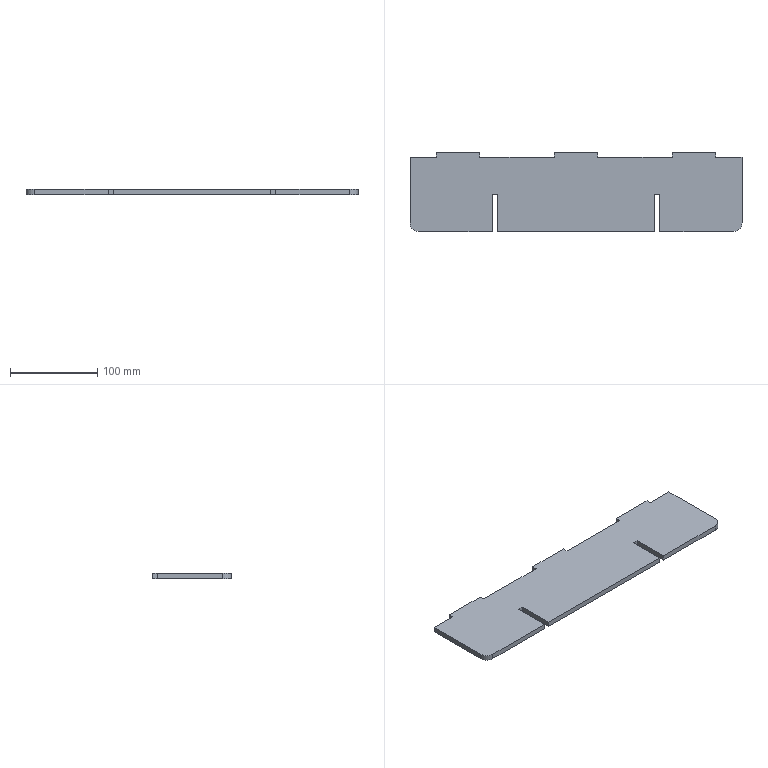Part | SolidWorks | features FlatPattern 1, SMBaseFlange 1, SheetMetal 1 | 1 solid | 28 faces | box 380 x 90.5 x 6 mm | volume 195432 mm3 | plane 26 | cylinder 2 | commonest cylinder face diameters 20 x2
STEP:
#1=CARTESIAN_POINT('',(-262.29,-508.5,0.));
#2=VERTEX_POINT('',#1);
#3=CARTESIAN_POINT('',(-262.29,-583.5,0.));
#4=VERTEX_POINT('',#3);
#5=CARTESIAN_POINT('',(-262.29,-508.5,0.));
#6=DIRECTION('',(0.,-1.,0.));
#7=VECTOR('',#6,1000.);
#8=LINE('',#5,#7);
#9=EDGE_CURVE('',#2,#4,#8,.T.);
#10=ORIENTED_EDGE('',*,*,#9,.F.);
#11=CARTESIAN_POINT('',(-262.29,-508.5,-6.));
#12=VERTEX_POINT('',#11);
#13=CARTESIAN_POINT('',(-262.29,-508.5,-6.));
#14=DIRECTION('',(0.,0.,1.));
#15=VECTOR('',#14,1000.);
#16=LINE('',#13,#15);
#17=EDGE_CURVE('',#12,#2,#16,.T.);
#18=ORIENTED_EDGE('',*,*,#17,.F.);
#19=CARTESIAN_POINT('',(-262.29,-583.5,-6.));
#20=VERTEX_POINT('',#19);
#21=CARTESIAN_POINT('',(-262.29,-508.5,-6.));
#22=DIRECTION('',(0.,-1.,0.));
#23=VECTOR('',#22,1000.);
#24=LINE('',#21,#23);
#25=EDGE_CURVE('',#12,#20,#24,.T.);
#26=ORIENTED_EDGE('',*,*,#25,.T.);
#27=CARTESIAN_POINT('',(-262.29,-583.5,-6.));
#28=DIRECTION('',(0.,0.,1.));
#29=VECTOR('',#28,1000.);
#30=LINE('',#27,#29);
#31=EDGE_CURVE('',#20,#4,#30,.T.);
#32=ORIENTED_EDGE('',*,*,#31,.T.);
#33=EDGE_LOOP('',(#10,#18,#26,#32));
#34=FACE_OUTER_BOUND('',#33,.T.);
#35=CARTESIAN_POINT('',(-262.29,-508.5,-6.));
#36=DIRECTION('',(-1.,0.,0.));
#37=DIRECTION('',(0.,0.,1.));
#38=AXIS2_PLACEMENT_3D('',#35,#36,#37);
#39=PLANE('',#38);
#40=ADVANCED_FACE('',(#34),#39,.T.);
#41=CARTESIAN_POINT('',(-232.29,-508.5,0.));
#42=VERTEX_POINT('',#41);
#43=CARTESIAN_POINT('',(-262.29,-508.5,0.));
#44=DIRECTION('',(-1.,0.,0.));
#45=VECTOR('',#44,1000.);
#46=LINE('',#43,#45);
#47=EDGE_CURVE('',#42,#2,#46,.T.);
#48=ORIENTED_EDGE('',*,*,#47,.F.);
#49=CARTESIAN_POINT('',(-232.29,-508.5,-6.));
#50=VERTEX_POINT('',#49);
#51=CARTESIAN_POINT('',(-232.29,-508.5,-6.));
#52=DIRECTION('',(0.,0.,1.));
#53=VECTOR('',#52,1000.);
#54=LINE('',#51,#53);
#55=EDGE_CURVE('',#50,#42,#54,.T.);
#56=ORIENTED_EDGE('',*,*,#55,.F.);
#57=CARTESIAN_POINT('',(-262.29,-508.5,-6.));
#58=DIRECTION('',(-1.,0.,0.));
#59=VECTOR('',#58,1000.);
#60=LINE('',#57,#59);
#61=EDGE_CURVE('',#50,#12,#60,.T.);
#62=ORIENTED_EDGE('',*,*,#61,.T.);
#63=ORIENTED_EDGE('',*,*,#17,.T.);
#64=EDGE_LOOP('',(#48,#56,#62,#63));
#65=FACE_OUTER_BOUND('',#64,.T.);
#66=CARTESIAN_POINT('',(-262.29,-508.5,-6.));
#67=DIRECTION('',(0.,1.,0.));
#68=DIRECTION('',(0.,0.,1.));
#69=AXIS2_PLACEMENT_3D('',#66,#67,#68);
#70=PLANE('',#69);
#71=ADVANCED_FACE('',(#65),#70,.T.);
#72=CARTESIAN_POINT('',(-232.29,-503.,0.));
#73=VERTEX_POINT('',#72);
#74=CARTESIAN_POINT('',(-232.29,-508.5,0.));
#75=DIRECTION('',(0.,-1.,0.));
#76=VECTOR('',#75,1000.);
#77=LINE('',#74,#76);
#78=EDGE_CURVE('',#73,#42,#77,.T.);
#79=ORIENTED_EDGE('',*,*,#78,.F.);
#80=CARTESIAN_POINT('',(-232.29,-503.,-6.));
#81=VERTEX_POINT('',#80);
#82=CARTESIAN_POINT('',(-232.29,-503.,-6.));
#83=DIRECTION('',(0.,0.,1.));
#84=VECTOR('',#83,1000.);
#85=LINE('',#82,#84);
#86=EDGE_CURVE('',#81,#73,#85,.T.);
#87=ORIENTED_EDGE('',*,*,#86,.F.);
#88=CARTESIAN_POINT('',(-232.29,-508.5,-6.));
#89=DIRECTION('',(0.,-1.,0.));
#90=VECTOR('',#89,1000.);
#91=LINE('',#88,#90);
#92=EDGE_CURVE('',#81,#50,#91,.T.);
#93=ORIENTED_EDGE('',*,*,#92,.T.);
#94=ORIENTED_EDGE('',*,*,#55,.T.);
#95=EDGE_LOOP('',(#79,#87,#93,#94));
#96=FACE_OUTER_BOUND('',#95,.T.);
#97=CARTESIAN_POINT('',(-232.29,-508.5,-6.));
#98=DIRECTION('',(-1.,0.,0.));
#99=DIRECTION('',(0.,0.,1.));
#100=AXIS2_PLACEMENT_3D('',#97,#98,#99);
#101=PLANE('',#100);
#102=ADVANCED_FACE('',(#96),#101,.T.);
#103=CARTESIAN_POINT('',(-182.29,-503.,0.));
#104=VERTEX_POINT('',#103);
#105=CARTESIAN_POINT('',(-232.29,-503.,0.));
#106=DIRECTION('',(-1.,0.,0.));
#107=VECTOR('',#106,1000.);
#108=LINE('',#105,#107);
#109=EDGE_CURVE('',#104,#73,#108,.T.);
#110=ORIENTED_EDGE('',*,*,#109,.F.);
#111=CARTESIAN_POINT('',(-182.29,-503.,-6.));
#112=VERTEX_POINT('',#111);
#113=CARTESIAN_POINT('',(-182.29,-503.,-6.));
#114=DIRECTION('',(0.,0.,1.));
#115=VECTOR('',#114,1000.);
#116=LINE('',#113,#115);
#117=EDGE_CURVE('',#112,#104,#116,.T.);
#118=ORIENTED_EDGE('',*,*,#117,.F.);
#119=CARTESIAN_POINT('',(-232.29,-503.,-6.));
#120=DIRECTION('',(-1.,0.,0.));
#121=VECTOR('',#120,1000.);
#122=LINE('',#119,#121);
#123=EDGE_CURVE('',#112,#81,#122,.T.);
#124=ORIENTED_EDGE('',*,*,#123,.T.);
#125=ORIENTED_EDGE('',*,*,#86,.T.);
#126=EDGE_LOOP('',(#110,#118,#124,#125));
#127=FACE_OUTER_BOUND('',#126,.T.);
#128=CARTESIAN_POINT('',(-232.29,-503.,-6.));
#129=DIRECTION('',(0.,1.,0.));
#130=DIRECTION('',(0.,0.,1.));
#131=AXIS2_PLACEMENT_3D('',#128,#129,#130);
#132=PLANE('',#131);
#133=ADVANCED_FACE('',(#127),#132,.T.);
#134=CARTESIAN_POINT('',(-182.29,-508.5,0.));
#135=VERTEX_POINT('',#134);
#136=CARTESIAN_POINT('',(-182.29,-503.,0.));
#137=DIRECTION('',(0.,1.,0.));
#138=VECTOR('',#137,1000.);
#139=LINE('',#136,#138);
#140=EDGE_CURVE('',#135,#104,#139,.T.);
#141=ORIENTED_EDGE('',*,*,#140,.F.);
#142=CARTESIAN_POINT('',(-182.29,-508.5,-6.));
#143=VERTEX_POINT('',#142);
#144=CARTESIAN_POINT('',(-182.29,-508.5,-6.));
#145=DIRECTION('',(0.,0.,1.));
#146=VECTOR('',#145,1000.);
#147=LINE('',#144,#146);
#148=EDGE_CURVE('',#143,#135,#147,.T.);
#149=ORIENTED_EDGE('',*,*,#148,.F.);
#150=CARTESIAN_POINT('',(-182.29,-503.,-6.));
#151=DIRECTION('',(0.,1.,0.));
#152=VECTOR('',#151,1000.);
#153=LINE('',#150,#152);
#154=EDGE_CURVE('',#143,#112,#153,.T.);
#155=ORIENTED_EDGE('',*,*,#154,.T.);
#156=ORIENTED_EDGE('',*,*,#117,.T.);
#157=EDGE_LOOP('',(#141,#149,#155,#156));
#158=FACE_OUTER_BOUND('',#157,.T.);
#159=CARTESIAN_POINT('',(-182.29,-503.,-6.));
#160=DIRECTION('',(1.,0.,0.));
#161=DIRECTION('',(0.,1.,0.));
#162=AXIS2_PLACEMENT_3D('',#159,#160,#161);
#163=PLANE('',#162);
#164=ADVANCED_FACE('',(#158),#163,.T.);
#165=CARTESIAN_POINT('',(-97.29,-508.5,0.));
#166=VERTEX_POINT('',#165);
#167=CARTESIAN_POINT('',(-182.29,-508.5,0.));
#168=DIRECTION('',(-1.,0.,0.));
#169=VECTOR('',#168,1000.);
#170=LINE('',#167,#169);
#171=EDGE_CURVE('',#166,#135,#170,.T.);
#172=ORIENTED_EDGE('',*,*,#171,.F.);
#173=CARTESIAN_POINT('',(-97.29,-508.5,-6.));
#174=VERTEX_POINT('',#173);
#175=CARTESIAN_POINT('',(-97.29,-508.5,-6.));
#176=DIRECTION('',(0.,0.,1.));
#177=VECTOR('',#176,1000.);
#178=LINE('',#175,#177);
#179=EDGE_CURVE('',#174,#166,#178,.T.);
#180=ORIENTED_EDGE('',*,*,#179,.F.);
#181=CARTESIAN_POINT('',(-182.29,-508.5,-6.));
#182=DIRECTION('',(-1.,0.,0.));
#183=VECTOR('',#182,1000.);
#184=LINE('',#181,#183);
#185=EDGE_CURVE('',#174,#143,#184,.T.);
#186=ORIENTED_EDGE('',*,*,#185,.T.);
#187=ORIENTED_EDGE('',*,*,#148,.T.);
#188=EDGE_LOOP('',(#172,#180,#186,#187));
#189=FACE_OUTER_BOUND('',#188,.T.);
#190=CARTESIAN_POINT('',(-182.29,-508.5,-6.));
#191=DIRECTION('',(0.,1.,0.));
#192=DIRECTION('',(0.,0.,1.));
#193=AXIS2_PLACEMENT_3D('',#190,#191,#192);
#194=PLANE('',#193);
#195=ADVANCED_FACE('',(#189),#194,.T.);
#196=CARTESIAN_POINT('',(-97.29,-503.,0.));
#197=VERTEX_POINT('',#196);
#198=CARTESIAN_POINT('',(-97.29,-508.5,0.));
#199=DIRECTION('',(0.,-1.,0.));
#200=VECTOR('',#199,1000.);
#201=LINE('',#198,#200);
#202=EDGE_CURVE('',#197,#166,#201,.T.);
#203=ORIENTED_EDGE('',*,*,#202,.F.);
#204=CARTESIAN_POINT('',(-97.29,-503.,-6.));
#205=VERTEX_POINT('',#204);
#206=CARTESIAN_POINT('',(-97.29,-503.,-6.));
#207=DIRECTION('',(0.,0.,1.));
#208=VECTOR('',#207,1000.);
#209=LINE('',#206,#208);
#210=EDGE_CURVE('',#205,#197,#209,.T.);
#211=ORIENTED_EDGE('',*,*,#210,.F.);
#212=CARTESIAN_POINT('',(-97.29,-508.5,-6.));
#213=DIRECTION('',(0.,-1.,0.));
#214=VECTOR('',#213,1000.);
#215=LINE('',#212,#214);
#216=EDGE_CURVE('',#205,#174,#215,.T.);
#217=ORIENTED_EDGE('',*,*,#216,.T.);
#218=ORIENTED_EDGE('',*,*,#179,.T.);
#219=EDGE_LOOP('',(#203,#211,#217,#218));
#220=FACE_OUTER_BOUND('',#219,.T.);
#221=CARTESIAN_POINT('',(-97.29,-508.5,-6.));
#222=DIRECTION('',(-1.,0.,0.));
#223=DIRECTION('',(0.,0.,1.));
#224=AXIS2_PLACEMENT_3D('',#221,#222,#223);
#225=PLANE('',#224);
#226=ADVANCED_FACE('',(#220),#225,.T.);
#227=CARTESIAN_POINT('',(-47.29,-503.,0.));
#228=VERTEX_POINT('',#227);
#229=CARTESIAN_POINT('',(-97.29,-503.,0.));
#230=DIRECTION('',(-1.,0.,0.));
#231=VECTOR('',#230,1000.);
#232=LINE('',#229,#231);
#233=EDGE_CURVE('',#228,#197,#232,.T.);
#234=ORIENTED_EDGE('',*,*,#233,.F.);
#235=CARTESIAN_POINT('',(-47.29,-503.,-6.));
#236=VERTEX_POINT('',#235);
#237=CARTESIAN_POINT('',(-47.29,-503.,-6.));
#238=DIRECTION('',(0.,0.,1.));
#239=VECTOR('',#238,1000.);
#240=LINE('',#237,#239);
#241=EDGE_CURVE('',#236,#228,#240,.T.);
#242=ORIENTED_EDGE('',*,*,#241,.F.);
#243=CARTESIAN_POINT('',(-97.29,-503.,-6.));
#244=DIRECTION('',(-1.,0.,0.));
#245=VECTOR('',#244,1000.);
#246=LINE('',#243,#245);
#247=EDGE_CURVE('',#236,#205,#246,.T.);
#248=ORIENTED_EDGE('',*,*,#247,.T.);
#249=ORIENTED_EDGE('',*,*,#210,.T.);
#250=EDGE_LOOP('',(#234,#242,#248,#249));
#251=FACE_OUTER_BOUND('',#250,.T.);
#252=CARTESIAN_POINT('',(-97.29,-503.,-6.));
#253=DIRECTION('',(0.,1.,0.));
#254=DIRECTION('',(0.,0.,1.));
#255=AXIS2_PLACEMENT_3D('',#252,#253,#254);
#256=PLANE('',#255);
#257=ADVANCED_FACE('',(#251),#256,.T.);
#258=CARTESIAN_POINT('',(-47.29,-508.5,0.));
#259=VERTEX_POINT('',#258);
#260=CARTESIAN_POINT('',(-47.29,-503.,0.));
#261=DIRECTION('',(0.,1.,0.));
#262=VECTOR('',#261,1000.);
#263=LINE('',#260,#262);
#264=EDGE_CURVE('',#259,#228,#263,.T.);
#265=ORIENTED_EDGE('',*,*,#264,.F.);
#266=CARTESIAN_POINT('',(-47.29,-508.5,-6.));
#267=VERTEX_POINT('',#266);
#268=CARTESIAN_POINT('',(-47.29,-508.5,-6.));
#269=DIRECTION('',(0.,0.,1.));
#270=VECTOR('',#269,1000.);
#271=LINE('',#268,#270);
#272=EDGE_CURVE('',#267,#259,#271,.T.);
#273=ORIENTED_EDGE('',*,*,#272,.F.);
#274=CARTESIAN_POINT('',(-47.29,-503.,-6.));
#275=DIRECTION('',(0.,1.,0.));
#276=VECTOR('',#275,1000.);
#277=LINE('',#274,#276);
#278=EDGE_CURVE('',#267,#236,#277,.T.);
#279=ORIENTED_EDGE('',*,*,#278,.T.);
#280=ORIENTED_EDGE('',*,*,#241,.T.);
#281=EDGE_LOOP('',(#265,#273,#279,#280));
#282=FACE_OUTER_BOUND('',#281,.T.);
#283=CARTESIAN_POINT('',(-47.29,-503.,-6.));
#284=DIRECTION('',(1.,0.,0.));
#285=DIRECTION('',(0.,0.,-1.));
#286=AXIS2_PLACEMENT_3D('',#283,#284,#285);
#287=PLANE('',#286);
#288=ADVANCED_FACE('',(#282),#287,.T.);
#289=CARTESIAN_POINT('',(37.71,-508.5,0.));
#290=VERTEX_POINT('',#289);
#291=CARTESIAN_POINT('',(-47.29,-508.5,0.));
#292=DIRECTION('',(-1.,0.,0.));
#293=VECTOR('',#292,1000.);
#294=LINE('',#291,#293);
#295=EDGE_CURVE('',#290,#259,#294,.T.);
#296=ORIENTED_EDGE('',*,*,#295,.F.);
#297=CARTESIAN_POINT('',(37.71,-508.5,-6.));
#298=VERTEX_POINT('',#297);
#299=CARTESIAN_POINT('',(37.71,-508.5,-6.));
#300=DIRECTION('',(0.,0.,1.));
#301=VECTOR('',#300,1000.);
#302=LINE('',#299,#301);
#303=EDGE_CURVE('',#298,#290,#302,.T.);
#304=ORIENTED_EDGE('',*,*,#303,.F.);
#305=CARTESIAN_POINT('',(-47.29,-508.5,-6.));
#306=DIRECTION('',(-1.,0.,0.));
#307=VECTOR('',#306,1000.);
#308=LINE('',#305,#307);
#309=EDGE_CURVE('',#298,#267,#308,.T.);
#310=ORIENTED_EDGE('',*,*,#309,.T.);
#311=ORIENTED_EDGE('',*,*,#272,.T.);
#312=EDGE_LOOP('',(#296,#304,#310,#311));
#313=FACE_OUTER_BOUND('',#312,.T.);
#314=CARTESIAN_POINT('',(-47.29,-508.5,-6.));
#315=DIRECTION('',(0.,1.,0.));
#316=DIRECTION('',(0.,0.,1.));
#317=AXIS2_PLACEMENT_3D('',#314,#315,#316);
#318=PLANE('',#317);
#319=ADVANCED_FACE('',(#313),#318,.T.);
#320=CARTESIAN_POINT('',(37.71,-503.,0.));
#321=VERTEX_POINT('',#320);
#322=CARTESIAN_POINT('',(37.71,-503.,0.));
#323=DIRECTION('',(0.,-1.,0.));
#324=VECTOR('',#323,1000.);
#325=LINE('',#322,#324);
#326=EDGE_CURVE('',#321,#290,#325,.T.);
#327=ORIENTED_EDGE('',*,*,#326,.F.);
#328=CARTESIAN_POINT('',(37.71,-503.,-6.));
#329=VERTEX_POINT('',#328);
#330=CARTESIAN_POINT('',(37.71,-503.,-6.));
#331=DIRECTION('',(0.,0.,1.));
#332=VECTOR('',#331,1000.);
#333=LINE('',#330,#332);
#334=EDGE_CURVE('',#329,#321,#333,.T.);
#335=ORIENTED_EDGE('',*,*,#334,.F.);
#336=CARTESIAN_POINT('',(37.71,-503.,-6.));
#337=DIRECTION('',(0.,-1.,0.));
#338=VECTOR('',#337,1000.);
#339=LINE('',#336,#338);
#340=EDGE_CURVE('',#329,#298,#339,.T.);
#341=ORIENTED_EDGE('',*,*,#340,.T.);
#342=ORIENTED_EDGE('',*,*,#303,.T.);
#343=EDGE_LOOP('',(#327,#335,#341,#342));
#344=FACE_OUTER_BOUND('',#343,.T.);
#345=CARTESIAN_POINT('',(37.71,-503.,-6.));
#346=DIRECTION('',(-1.,0.,0.));
#347=DIRECTION('',(0.,-1.,0.));
#348=AXIS2_PLACEMENT_3D('',#345,#346,#347);
#349=PLANE('',#348);
#350=ADVANCED_FACE('',(#344),#349,.T.);
#351=CARTESIAN_POINT('',(87.71,-503.,0.));
#352=VERTEX_POINT('',#351);
#353=CARTESIAN_POINT('',(87.71,-503.,0.));
#354=DIRECTION('',(-1.,0.,0.));
#355=VECTOR('',#354,1000.);
#356=LINE('',#353,#355);
#357=EDGE_CURVE('',#352,#321,#356,.T.);
#358=ORIENTED_EDGE('',*,*,#357,.F.);
#359=CARTESIAN_POINT('',(87.71,-503.,-6.));
#360=VERTEX_POINT('',#359);
#361=CARTESIAN_POINT('',(87.71,-503.,-6.));
#362=DIRECTION('',(0.,0.,1.));
#363=VECTOR('',#362,1000.);
#364=LINE('',#361,#363);
#365=EDGE_CURVE('',#360,#352,#364,.T.);
#366=ORIENTED_EDGE('',*,*,#365,.F.);
#367=CARTESIAN_POINT('',(87.71,-503.,-6.));
#368=DIRECTION('',(-1.,0.,0.));
#369=VECTOR('',#368,1000.);
#370=LINE('',#367,#369);
#371=EDGE_CURVE('',#360,#329,#370,.T.);
#372=ORIENTED_EDGE('',*,*,#371,.T.);
#373=ORIENTED_EDGE('',*,*,#334,.T.);
#374=EDGE_LOOP('',(#358,#366,#372,#373));
#375=FACE_OUTER_BOUND('',#374,.T.);
#376=CARTESIAN_POINT('',(87.71,-503.,-6.));
#377=DIRECTION('',(0.,1.,0.));
#378=DIRECTION('',(0.,0.,1.));
#379=AXIS2_PLACEMENT_3D('',#376,#377,#378);
#380=PLANE('',#379);
#381=ADVANCED_FACE('',(#375),#380,.T.);
#382=CARTESIAN_POINT('',(87.71,-508.5,0.));
#383=VERTEX_POINT('',#382);
#384=CARTESIAN_POINT('',(87.71,-508.5,0.));
#385=DIRECTION('',(0.,1.,0.));
#386=VECTOR('',#385,1000.);
#387=LINE('',#384,#386);
#388=EDGE_CURVE('',#383,#352,#387,.T.);
#389=ORIENTED_EDGE('',*,*,#388,.F.);
#390=CARTESIAN_POINT('',(87.71,-508.5,-6.));
#391=VERTEX_POINT('',#390);
#392=CARTESIAN_POINT('',(87.71,-508.5,-6.));
#393=DIRECTION('',(0.,0.,1.));
#394=VECTOR('',#393,1000.);
#395=LINE('',#392,#394);
#396=EDGE_CURVE('',#391,#383,#395,.T.);
#397=ORIENTED_EDGE('',*,*,#396,.F.);
#398=CARTESIAN_POINT('',(87.71,-508.5,-6.));
#399=DIRECTION('',(0.,1.,0.));
#400=VECTOR('',#399,1000.);
#401=LINE('',#398,#400);
#402=EDGE_CURVE('',#391,#360,#401,.T.);
#403=ORIENTED_EDGE('',*,*,#402,.T.);
#404=ORIENTED_EDGE('',*,*,#365,.T.);
#405=EDGE_LOOP('',(#389,#397,#403,#404));
#406=FACE_OUTER_BOUND('',#405,.T.);
#407=CARTESIAN_POINT('',(87.71,-508.5,-6.));
#408=DIRECTION('',(1.,0.,0.));
#409=DIRECTION('',(0.,0.,-1.));
#410=AXIS2_PLACEMENT_3D('',#407,#408,#409);
#411=PLANE('',#410);
#412=ADVANCED_FACE('',(#406),#411,.T.);
#413=CARTESIAN_POINT('',(117.71,-508.5,0.));
#414=VERTEX_POINT('',#413);
#415=CARTESIAN_POINT('',(87.71,-508.5,0.));
#416=DIRECTION('',(-1.,0.,0.));
#417=VECTOR('',#416,1000.);
#418=LINE('',#415,#417);
#419=EDGE_CURVE('',#414,#383,#418,.T.);
#420=ORIENTED_EDGE('',*,*,#419,.F.);
#421=CARTESIAN_POINT('',(117.71,-508.5,-6.));
#422=VERTEX_POINT('',#421);
#423=CARTESIAN_POINT('',(117.71,-508.5,-6.));
#424=DIRECTION('',(0.,0.,1.));
#425=VECTOR('',#424,1000.);
#426=LINE('',#423,#425);
#427=EDGE_CURVE('',#422,#414,#426,.T.);
#428=ORIENTED_EDGE('',*,*,#427,.F.);
#429=CARTESIAN_POINT('',(87.71,-508.5,-6.));
#430=DIRECTION('',(-1.,0.,0.));
#431=VECTOR('',#430,1000.);
#432=LINE('',#429,#431);
#433=EDGE_CURVE('',#422,#391,#432,.T.);
#434=ORIENTED_EDGE('',*,*,#433,.T.);
#435=ORIENTED_EDGE('',*,*,#396,.T.);
#436=EDGE_LOOP('',(#420,#428,#434,#435));
#437=FACE_OUTER_BOUND('',#436,.T.);
#438=CARTESIAN_POINT('',(87.71,-508.5,-6.));
#439=DIRECTION('',(0.,1.,0.));
#440=DIRECTION('',(0.,0.,1.));
#441=AXIS2_PLACEMENT_3D('',#438,#439,#440);
#442=PLANE('',#441);
#443=ADVANCED_FACE('',(#437),#442,.T.);
#444=CARTESIAN_POINT('',(117.71,-583.5,0.));
#445=VERTEX_POINT('',#444);
#446=CARTESIAN_POINT('',(117.71,-508.5,0.));
#447=DIRECTION('',(0.,1.,0.));
#448=VECTOR('',#447,1000.);
#449=LINE('',#446,#448);
#450=EDGE_CURVE('',#445,#414,#449,.T.);
#451=ORIENTED_EDGE('',*,*,#450,.F.);
#452=CARTESIAN_POINT('',(117.71,-583.5,-6.));
#453=VERTEX_POINT('',#452);
#454=CARTESIAN_POINT('',(117.71,-583.5,-6.));
#455=DIRECTION('',(0.,0.,1.));
#456=VECTOR('',#455,1000.);
#457=LINE('',#454,#456);
#458=EDGE_CURVE('',#453,#445,#457,.T.);
#459=ORIENTED_EDGE('',*,*,#458,.F.);
#460=CARTESIAN_POINT('',(117.71,-508.5,-6.));
#461=DIRECTION('',(0.,1.,0.));
#462=VECTOR('',#461,1000.);
#463=LINE('',#460,#462);
#464=EDGE_CURVE('',#453,#422,#463,.T.);
#465=ORIENTED_EDGE('',*,*,#464,.T.);
#466=ORIENTED_EDGE('',*,*,#427,.T.);
#467=EDGE_LOOP('',(#451,#459,#465,#466));
#468=FACE_OUTER_BOUND('',#467,.T.);
#469=CARTESIAN_POINT('',(117.71,-508.5,-6.));
#470=DIRECTION('',(1.,0.,0.));
#471=DIRECTION('',(0.,0.,-1.));
#472=AXIS2_PLACEMENT_3D('',#469,#470,#471);
#473=PLANE('',#472);
#474=ADVANCED_FACE('',(#468),#473,.T.);
#475=CARTESIAN_POINT('',(107.71,-593.5,0.));
#476=VERTEX_POINT('',#475);
#477=CARTESIAN_POINT('',(107.71,-583.5,0.));
#478=DIRECTION('',(0.,0.,1.));
#479=DIRECTION('',(1.,0.,0.));
#480=AXIS2_PLACEMENT_3D('',#477,#478,#479);
#481=CIRCLE('',#480,10.);
#482=EDGE_CURVE('',#476,#445,#481,.T.);
#483=ORIENTED_EDGE('',*,*,#482,.F.);
#484=CARTESIAN_POINT('',(107.71,-593.5,-6.));
#485=VERTEX_POINT('',#484);
#486=CARTESIAN_POINT('',(107.71,-593.5,-6.));
#487=DIRECTION('',(0.,0.,1.));
#488=VECTOR('',#487,1000.);
#489=LINE('',#486,#488);
#490=EDGE_CURVE('',#485,#476,#489,.T.);
#491=ORIENTED_EDGE('',*,*,#490,.F.);
#492=CARTESIAN_POINT('',(107.71,-583.5,-6.));
#493=DIRECTION('',(0.,0.,1.));
#494=DIRECTION('',(1.,0.,0.));
#495=AXIS2_PLACEMENT_3D('',#492,#493,#494);
#496=CIRCLE('',#495,10.);
#497=EDGE_CURVE('',#485,#453,#496,.T.);
#498=ORIENTED_EDGE('',*,*,#497,.T.);
#499=ORIENTED_EDGE('',*,*,#458,.T.);
#500=EDGE_LOOP('',(#483,#491,#498,#499));
#501=FACE_OUTER_BOUND('',#500,.T.);
#502=CARTESIAN_POINT('',(107.71,-583.5,-6.));
#503=DIRECTION('',(0.,0.,1.));
#504=DIRECTION('',(1.,0.,0.));
#505=AXIS2_PLACEMENT_3D('',#502,#503,#504);
#506=CYLINDRICAL_SURFACE('',#505,10.);
#507=ADVANCED_FACE('',(#501),#506,.T.);
#508=CARTESIAN_POINT('',(23.71,-593.5,0.));
#509=VERTEX_POINT('',#508);
#510=CARTESIAN_POINT('',(23.71,-593.5,0.));
#511=DIRECTION('',(1.,0.,0.));
#512=VECTOR('',#511,1000.);
#513=LINE('',#510,#512);
#514=EDGE_CURVE('',#509,#476,#513,.T.);
#515=ORIENTED_EDGE('',*,*,#514,.F.);
#516=CARTESIAN_POINT('',(23.71,-593.5,-6.));
#517=VERTEX_POINT('',#516);
#518=CARTESIAN_POINT('',(23.71,-593.5,-6.));
#519=DIRECTION('',(0.,0.,1.));
#520=VECTOR('',#519,1000.);
#521=LINE('',#518,#520);
#522=EDGE_CURVE('',#517,#509,#521,.T.);
#523=ORIENTED_EDGE('',*,*,#522,.F.);
#524=CARTESIAN_POINT('',(23.71,-593.5,-6.));
#525=DIRECTION('',(1.,0.,0.));
#526=VECTOR('',#525,1000.);
#527=LINE('',#524,#526);
#528=EDGE_CURVE('',#517,#485,#527,.T.);
#529=ORIENTED_EDGE('',*,*,#528,.T.);
#530=ORIENTED_EDGE('',*,*,#490,.T.);
#531=EDGE_LOOP('',(#515,#523,#529,#530));
#532=FACE_OUTER_BOUND('',#531,.T.);
#533=CARTESIAN_POINT('',(23.71,-593.5,-6.));
#534=DIRECTION('',(0.,-1.,0.));
#535=DIRECTION('',(0.,0.,-1.));
#536=AXIS2_PLACEMENT_3D('',#533,#534,#535);
#537=PLANE('',#536);
#538=ADVANCED_FACE('',(#532),#537,.T.);
#539=CARTESIAN_POINT('',(23.71,-551.,0.));
#540=VERTEX_POINT('',#539);
#541=CARTESIAN_POINT('',(23.71,-593.5,0.));
#542=DIRECTION('',(0.,-1.,0.));
#543=VECTOR('',#542,1000.);
#544=LINE('',#541,#543);
#545=EDGE_CURVE('',#540,#509,#544,.T.);
#546=ORIENTED_EDGE('',*,*,#545,.F.);
#547=CARTESIAN_POINT('',(23.71,-551.,-6.));
#548=VERTEX_POINT('',#547);
#549=CARTESIAN_POINT('',(23.71,-551.,-6.));
#550=DIRECTION('',(0.,0.,1.));
#551=VECTOR('',#550,1000.);
#552=LINE('',#549,#551);
#553=EDGE_CURVE('',#548,#540,#552,.T.);
#554=ORIENTED_EDGE('',*,*,#553,.F.);
#555=CARTESIAN_POINT('',(23.71,-593.5,-6.));
#556=DIRECTION('',(0.,-1.,0.));
#557=VECTOR('',#556,1000.);
#558=LINE('',#555,#557);
#559=EDGE_CURVE('',#548,#517,#558,.T.);
#560=ORIENTED_EDGE('',*,*,#559,.T.);
#561=ORIENTED_EDGE('',*,*,#522,.T.);
#562=EDGE_LOOP('',(#546,#554,#560,#561));
#563=FACE_OUTER_BOUND('',#562,.T.);
#564=CARTESIAN_POINT('',(23.71,-593.5,-6.));
#565=DIRECTION('',(-1.,0.,0.));
#566=DIRECTION('',(0.,0.,1.));
#567=AXIS2_PLACEMENT_3D('',#564,#565,#566);
#568=PLANE('',#567);
#569=ADVANCED_FACE('',(#563),#568,.T.);
#570=CARTESIAN_POINT('',(17.71,-551.,0.));
#571=VERTEX_POINT('',#570);
#572=CARTESIAN_POINT('',(23.71,-551.,0.));
#573=DIRECTION('',(1.,0.,0.));
#574=VECTOR('',#573,1000.);
#575=LINE('',#572,#574);
#576=EDGE_CURVE('',#571,#540,#575,.T.);
#577=ORIENTED_EDGE('',*,*,#576,.F.);
#578=CARTESIAN_POINT('',(17.71,-551.,-6.));
#579=VERTEX_POINT('',#578);
#580=CARTESIAN_POINT('',(17.71,-551.,-6.));
#581=DIRECTION('',(0.,0.,1.));
#582=VECTOR('',#581,1000.);
#583=LINE('',#580,#582);
#584=EDGE_CURVE('',#579,#571,#583,.T.);
#585=ORIENTED_EDGE('',*,*,#584,.F.);
#586=CARTESIAN_POINT('',(23.71,-551.,-6.));
#587=DIRECTION('',(1.,0.,0.));
#588=VECTOR('',#587,1000.);
#589=LINE('',#586,#588);
#590=EDGE_CURVE('',#579,#548,#589,.T.);
#591=ORIENTED_EDGE('',*,*,#590,.T.);
#592=ORIENTED_EDGE('',*,*,#553,.T.);
#593=EDGE_LOOP('',(#577,#585,#591,#592));
#594=FACE_OUTER_BOUND('',#593,.T.);
#595=CARTESIAN_POINT('',(23.71,-551.,-6.));
#596=DIRECTION('',(0.,-1.,0.));
#597=DIRECTION('',(0.,0.,-1.));
#598=AXIS2_PLACEMENT_3D('',#595,#596,#597);
#599=PLANE('',#598);
#600=ADVANCED_FACE('',(#594),#599,.T.);
#601=CARTESIAN_POINT('',(17.71,-593.5,0.));
#602=VERTEX_POINT('',#601);
#603=CARTESIAN_POINT('',(17.71,-551.,0.));
#604=DIRECTION('',(0.,1.,0.));
#605=VECTOR('',#604,1000.);
#606=LINE('',#603,#605);
#607=EDGE_CURVE('',#602,#571,#606,.T.);
#608=ORIENTED_EDGE('',*,*,#607,.F.);
#609=CARTESIAN_POINT('',(17.71,-593.5,-6.));
#610=VERTEX_POINT('',#609);
#611=CARTESIAN_POINT('',(17.71,-593.5,-6.));
#612=DIRECTION('',(0.,0.,1.));
#613=VECTOR('',#612,1000.);
#614=LINE('',#611,#613);
#615=EDGE_CURVE('',#610,#602,#614,.T.);
#616=ORIENTED_EDGE('',*,*,#615,.F.);
#617=CARTESIAN_POINT('',(17.71,-551.,-6.));
#618=DIRECTION('',(0.,1.,0.));
#619=VECTOR('',#618,1000.);
#620=LINE('',#617,#619);
#621=EDGE_CURVE('',#610,#579,#620,.T.);
#622=ORIENTED_EDGE('',*,*,#621,.T.);
#623=ORIENTED_EDGE('',*,*,#584,.T.);
#624=EDGE_LOOP('',(#608,#616,#622,#623));
#625=FACE_OUTER_BOUND('',#624,.T.);
#626=CARTESIAN_POINT('',(17.71,-551.,-6.));
#627=DIRECTION('',(1.,0.,0.));
#628=DIRECTION('',(0.,0.,-1.));
#629=AXIS2_PLACEMENT_3D('',#626,#627,#628);
#630=PLANE('',#629);
#631=ADVANCED_FACE('',(#625),#630,.T.);
#632=CARTESIAN_POINT('',(-162.29,-593.5,0.));
#633=VERTEX_POINT('',#632);
#634=CARTESIAN_POINT('',(-162.29,-593.5,0.));
#635=DIRECTION('',(1.,0.,0.));
#636=VECTOR('',#635,1000.);
#637=LINE('',#634,#636);
#638=EDGE_CURVE('',#633,#602,#637,.T.);
#639=ORIENTED_EDGE('',*,*,#638,.F.);
#640=CARTESIAN_POINT('',(-162.29,-593.5,-6.));
#641=VERTEX_POINT('',#640);
#642=CARTESIAN_POINT('',(-162.29,-593.5,-6.));
#643=DIRECTION('',(0.,0.,1.));
#644=VECTOR('',#643,1000.);
#645=LINE('',#642,#644);
#646=EDGE_CURVE('',#641,#633,#645,.T.);
#647=ORIENTED_EDGE('',*,*,#646,.F.);
#648=CARTESIAN_POINT('',(-162.29,-593.5,-6.));
#649=DIRECTION('',(1.,0.,0.));
#650=VECTOR('',#649,1000.);
#651=LINE('',#648,#650);
#652=EDGE_CURVE('',#641,#610,#651,.T.);
#653=ORIENTED_EDGE('',*,*,#652,.T.);
#654=ORIENTED_EDGE('',*,*,#615,.T.);
#655=EDGE_LOOP('',(#639,#647,#653,#654));
#656=FACE_OUTER_BOUND('',#655,.T.);
#657=CARTESIAN_POINT('',(-162.29,-593.5,-6.));
#658=DIRECTION('',(0.,-1.,0.));
#659=DIRECTION('',(0.,0.,-1.));
#660=AXIS2_PLACEMENT_3D('',#657,#658,#659);
#661=PLANE('',#660);
#662=ADVANCED_FACE('',(#656),#661,.T.);
#663=CARTESIAN_POINT('',(-162.29,-551.,0.));
#664=VERTEX_POINT('',#663);
#665=CARTESIAN_POINT('',(-162.29,-593.5,0.));
#666=DIRECTION('',(0.,-1.,0.));
#667=VECTOR('',#666,1000.);
#668=LINE('',#665,#667);
#669=EDGE_CURVE('',#664,#633,#668,.T.);
#670=ORIENTED_EDGE('',*,*,#669,.F.);
#671=CARTESIAN_POINT('',(-162.29,-551.,-6.));
#672=VERTEX_POINT('',#671);
#673=CARTESIAN_POINT('',(-162.29,-551.,-6.));
#674=DIRECTION('',(0.,0.,1.));
#675=VECTOR('',#674,1000.);
#676=LINE('',#673,#675);
#677=EDGE_CURVE('',#672,#664,#676,.T.);
#678=ORIENTED_EDGE('',*,*,#677,.F.);
#679=CARTESIAN_POINT('',(-162.29,-593.5,-6.));
#680=DIRECTION('',(0.,-1.,0.));
#681=VECTOR('',#680,1000.);
#682=LINE('',#679,#681);
#683=EDGE_CURVE('',#672,#641,#682,.T.);
#684=ORIENTED_EDGE('',*,*,#683,.T.);
#685=ORIENTED_EDGE('',*,*,#646,.T.);
#686=EDGE_LOOP('',(#670,#678,#684,#685));
#687=FACE_OUTER_BOUND('',#686,.T.);
#688=CARTESIAN_POINT('',(-162.29,-593.5,-6.));
#689=DIRECTION('',(-1.,0.,0.));
#690=DIRECTION('',(0.,0.,1.));
#691=AXIS2_PLACEMENT_3D('',#688,#689,#690);
#692=PLANE('',#691);
#693=ADVANCED_FACE('',(#687),#692,.T.);
#694=CARTESIAN_POINT('',(-168.29,-551.,0.));
#695=VERTEX_POINT('',#694);
#696=CARTESIAN_POINT('',(-162.29,-551.,0.));
#697=DIRECTION('',(1.,0.,0.));
#698=VECTOR('',#697,1000.);
#699=LINE('',#696,#698);
#700=EDGE_CURVE('',#695,#664,#699,.T.);
#701=ORIENTED_EDGE('',*,*,#700,.F.);
#702=CARTESIAN_POINT('',(-168.29,-551.,-6.));
#703=VERTEX_POINT('',#702);
#704=CARTESIAN_POINT('',(-168.29,-551.,-6.));
#705=DIRECTION('',(0.,0.,1.));
#706=VECTOR('',#705,1000.);
#707=LINE('',#704,#706);
#708=EDGE_CURVE('',#703,#695,#707,.T.);
#709=ORIENTED_EDGE('',*,*,#708,.F.);
#710=CARTESIAN_POINT('',(-162.29,-551.,-6.));
#711=DIRECTION('',(1.,0.,0.));
#712=VECTOR('',#711,1000.);
#713=LINE('',#710,#712);
#714=EDGE_CURVE('',#703,#672,#713,.T.);
#715=ORIENTED_EDGE('',*,*,#714,.T.);
#716=ORIENTED_EDGE('',*,*,#677,.T.);
#717=EDGE_LOOP('',(#701,#709,#715,#716));
#718=FACE_OUTER_BOUND('',#717,.T.);
#719=CARTESIAN_POINT('',(-162.29,-551.,-6.));
#720=DIRECTION('',(0.,-1.,0.));
#721=DIRECTION('',(0.,0.,-1.));
#722=AXIS2_PLACEMENT_3D('',#719,#720,#721);
#723=PLANE('',#722);
#724=ADVANCED_FACE('',(#718),#723,.T.);
#725=CARTESIAN_POINT('',(-168.29,-593.5,0.));
#726=VERTEX_POINT('',#725);
#727=CARTESIAN_POINT('',(-168.29,-551.,0.));
#728=DIRECTION('',(0.,1.,0.));
#729=VECTOR('',#728,1000.);
#730=LINE('',#727,#729);
#731=EDGE_CURVE('',#726,#695,#730,.T.);
#732=ORIENTED_EDGE('',*,*,#731,.F.);
#733=CARTESIAN_POINT('',(-168.29,-593.5,-6.));
#734=VERTEX_POINT('',#733);
#735=CARTESIAN_POINT('',(-168.29,-593.5,-6.));
#736=DIRECTION('',(0.,0.,1.));
#737=VECTOR('',#736,1000.);
#738=LINE('',#735,#737);
#739=EDGE_CURVE('',#734,#726,#738,.T.);
#740=ORIENTED_EDGE('',*,*,#739,.F.);
#741=CARTESIAN_POINT('',(-168.29,-551.,-6.));
#742=DIRECTION('',(0.,1.,0.));
#743=VECTOR('',#742,1000.);
#744=LINE('',#741,#743);
#745=EDGE_CURVE('',#734,#703,#744,.T.);
#746=ORIENTED_EDGE('',*,*,#745,.T.);
#747=ORIENTED_EDGE('',*,*,#708,.T.);
#748=EDGE_LOOP('',(#732,#740,#746,#747));
#749=FACE_OUTER_BOUND('',#748,.T.);
#750=CARTESIAN_POINT('',(-168.29,-551.,-6.));
#751=DIRECTION('',(1.,0.,0.));
#752=DIRECTION('',(0.,0.,-1.));
#753=AXIS2_PLACEMENT_3D('',#750,#751,#752);
#754=PLANE('',#753);
#755=ADVANCED_FACE('',(#749),#754,.T.);
#756=CARTESIAN_POINT('',(-252.29,-593.5,0.));
#757=VERTEX_POINT('',#756);
#758=CARTESIAN_POINT('',(-252.29,-593.5,0.));
#759=DIRECTION('',(1.,0.,0.));
#760=VECTOR('',#759,1000.);
#761=LINE('',#758,#760);
#762=EDGE_CURVE('',#757,#726,#761,.T.);
#763=ORIENTED_EDGE('',*,*,#762,.F.);
#764=CARTESIAN_POINT('',(-252.29,-593.5,-6.));
#765=VERTEX_POINT('',#764);
#766=CARTESIAN_POINT('',(-252.29,-593.5,-6.));
#767=DIRECTION('',(0.,0.,1.));
#768=VECTOR('',#767,1000.);
#769=LINE('',#766,#768);
#770=EDGE_CURVE('',#765,#757,#769,.T.);
#771=ORIENTED_EDGE('',*,*,#770,.F.);
#772=CARTESIAN_POINT('',(-252.29,-593.5,-6.));
#773=DIRECTION('',(1.,0.,0.));
#774=VECTOR('',#773,1000.);
#775=LINE('',#772,#774);
#776=EDGE_CURVE('',#765,#734,#775,.T.);
#777=ORIENTED_EDGE('',*,*,#776,.T.);
#778=ORIENTED_EDGE('',*,*,#739,.T.);
#779=EDGE_LOOP('',(#763,#771,#777,#778));
#780=FACE_OUTER_BOUND('',#779,.T.);
#781=CARTESIAN_POINT('',(-252.29,-593.5,-6.));
#782=DIRECTION('',(0.,-1.,0.));
#783=DIRECTION('',(0.,0.,-1.));
#784=AXIS2_PLACEMENT_3D('',#781,#782,#783);
#785=PLANE('',#784);
#786=ADVANCED_FACE('',(#780),#785,.T.);
#787=CARTESIAN_POINT('',(-252.29,-583.5,0.));
#788=DIRECTION('',(0.,0.,1.));
#789=DIRECTION('',(1.,0.,0.));
#790=AXIS2_PLACEMENT_3D('',#787,#788,#789);
#791=CIRCLE('',#790,10.);
#792=EDGE_CURVE('',#4,#757,#791,.T.);
#793=ORIENTED_EDGE('',*,*,#792,.F.);
#794=ORIENTED_EDGE('',*,*,#31,.F.);
#795=CARTESIAN_POINT('',(-252.29,-583.5,-6.));
#796=DIRECTION('',(0.,0.,1.));
#797=DIRECTION('',(1.,0.,0.));
#798=AXIS2_PLACEMENT_3D('',#795,#796,#797);
#799=CIRCLE('',#798,10.);
#800=EDGE_CURVE('',#20,#765,#799,.T.);
#801=ORIENTED_EDGE('',*,*,#800,.T.);
#802=ORIENTED_EDGE('',*,*,#770,.T.);
#803=EDGE_LOOP('',(#793,#794,#801,#802));
#804=FACE_OUTER_BOUND('',#803,.T.);
#805=CARTESIAN_POINT('',(-252.29,-583.5,-6.));
#806=DIRECTION('',(0.,0.,1.));
#807=DIRECTION('',(1.,0.,0.));
#808=AXIS2_PLACEMENT_3D('',#805,#806,#807);
#809=CYLINDRICAL_SURFACE('',#808,10.);
#810=ADVANCED_FACE('',(#804),#809,.T.);
#811=ORIENTED_EDGE('',*,*,#25,.F.);
#812=ORIENTED_EDGE('',*,*,#61,.F.);
#813=ORIENTED_EDGE('',*,*,#92,.F.);
#814=ORIENTED_EDGE('',*,*,#123,.F.);
#815=ORIENTED_EDGE('',*,*,#154,.F.);
#816=ORIENTED_EDGE('',*,*,#185,.F.);
#817=ORIENTED_EDGE('',*,*,#216,.F.);
#818=ORIENTED_EDGE('',*,*,#247,.F.);
#819=ORIENTED_EDGE('',*,*,#278,.F.);
#820=ORIENTED_EDGE('',*,*,#309,.F.);
#821=ORIENTED_EDGE('',*,*,#340,.F.);
#822=ORIENTED_EDGE('',*,*,#371,.F.);
#823=ORIENTED_EDGE('',*,*,#402,.F.);
#824=ORIENTED_EDGE('',*,*,#433,.F.);
#825=ORIENTED_EDGE('',*,*,#464,.F.);
#826=ORIENTED_EDGE('',*,*,#497,.F.);
#827=ORIENTED_EDGE('',*,*,#528,.F.);
#828=ORIENTED_EDGE('',*,*,#559,.F.);
#829=ORIENTED_EDGE('',*,*,#590,.F.);
#830=ORIENTED_EDGE('',*,*,#621,.F.);
#831=ORIENTED_EDGE('',*,*,#652,.F.);
#832=ORIENTED_EDGE('',*,*,#683,.F.);
#833=ORIENTED_EDGE('',*,*,#714,.F.);
#834=ORIENTED_EDGE('',*,*,#745,.F.);
#835=ORIENTED_EDGE('',*,*,#776,.F.);
#836=ORIENTED_EDGE('',*,*,#800,.F.);
#837=EDGE_LOOP('',(#811,#812,#813,#814,#815,#816,#817,#818,#819,#820,#821,#822,#823,#824,#825,#826,#827,#828,#829,#830,#831,#832,#833,#834,#835,#836));
#838=FACE_OUTER_BOUND('',#837,.T.);
#839=CARTESIAN_POINT('',(-252.29,-583.5,-6.));
#840=DIRECTION('',(0.,0.,1.));
#841=DIRECTION('',(1.,0.,0.));
#842=AXIS2_PLACEMENT_3D('',#839,#840,#841);
#843=PLANE('',#842);
#844=ADVANCED_FACE('',(#838),#843,.F.);
#845=ORIENTED_EDGE('',*,*,#9,.T.);
#846=ORIENTED_EDGE('',*,*,#792,.T.);
#847=ORIENTED_EDGE('',*,*,#762,.T.);
#848=ORIENTED_EDGE('',*,*,#731,.T.);
#849=ORIENTED_EDGE('',*,*,#700,.T.);
#850=ORIENTED_EDGE('',*,*,#669,.T.);
#851=ORIENTED_EDGE('',*,*,#638,.T.);
#852=ORIENTED_EDGE('',*,*,#607,.T.);
#853=ORIENTED_EDGE('',*,*,#576,.T.);
#854=ORIENTED_EDGE('',*,*,#545,.T.);
#855=ORIENTED_EDGE('',*,*,#514,.T.);
#856=ORIENTED_EDGE('',*,*,#482,.T.);
#857=ORIENTED_EDGE('',*,*,#450,.T.);
#858=ORIENTED_EDGE('',*,*,#419,.T.);
#859=ORIENTED_EDGE('',*,*,#388,.T.);
#860=ORIENTED_EDGE('',*,*,#357,.T.);
#861=ORIENTED_EDGE('',*,*,#326,.T.);
#862=ORIENTED_EDGE('',*,*,#295,.T.);
#863=ORIENTED_EDGE('',*,*,#264,.T.);
#864=ORIENTED_EDGE('',*,*,#233,.T.);
#865=ORIENTED_EDGE('',*,*,#202,.T.);
#866=ORIENTED_EDGE('',*,*,#171,.T.);
#867=ORIENTED_EDGE('',*,*,#140,.T.);
#868=ORIENTED_EDGE('',*,*,#109,.T.);
#869=ORIENTED_EDGE('',*,*,#78,.T.);
#870=ORIENTED_EDGE('',*,*,#47,.T.);
#871=EDGE_LOOP('',(#845,#846,#847,#848,#849,#850,#851,#852,#853,#854,#855,#856,#857,#858,#859,#860,#861,#862,#863,#864,#865,#866,#867,#868,#869,#870));
#872=FACE_OUTER_BOUND('',#871,.T.);
#873=CARTESIAN_POINT('',(-252.29,-583.5,0.));
#874=DIRECTION('',(0.,0.,1.));
#875=DIRECTION('',(1.,0.,0.));
#876=AXIS2_PLACEMENT_3D('',#873,#874,#875);
#877=PLANE('',#876);
#878=ADVANCED_FACE('',(#872),#877,.T.);
#879=CLOSED_SHELL('',(#40,#71,#102,#133,#164,#195,#226,#257,#288,#319,#350,#381,#412,#443,#474,#507,#538,#569,#600,#631,#662,#693,#724,#755,#786,#810,#844,#878));
#880=MANIFOLD_SOLID_BREP('',#879);
#881=CARTESIAN_POINT('',(0.,0.,0.));
#882=DIRECTION('',(0.,0.,1.));
#883=DIRECTION('',(1.,0.,0.));
#884=AXIS2_PLACEMENT_3D('',#881,#882,#883);
#885=(LENGTH_UNIT()NAMED_UNIT(*)SI_UNIT(.MILLI.,.METRE.));
#886=UNCERTAINTY_MEASURE_WITH_UNIT(LENGTH_MEASURE(0.00001),#885,'','');
#887=(NAMED_UNIT(*)PLANE_ANGLE_UNIT()SI_UNIT($,.RADIAN.));
#888=(NAMED_UNIT(*)SI_UNIT($,.STERADIAN.)SOLID_ANGLE_UNIT());
#889=(GEOMETRIC_REPRESENTATION_CONTEXT(3)GLOBAL_UNCERTAINTY_ASSIGNED_CONTEXT((#886))GLOBAL_UNIT_ASSIGNED_CONTEXT((#885,#887,#888))REPRESENTATION_CONTEXT('',''));
#890=ADVANCED_BREP_SHAPE_REPRESENTATION('',(#880,#884),#889);